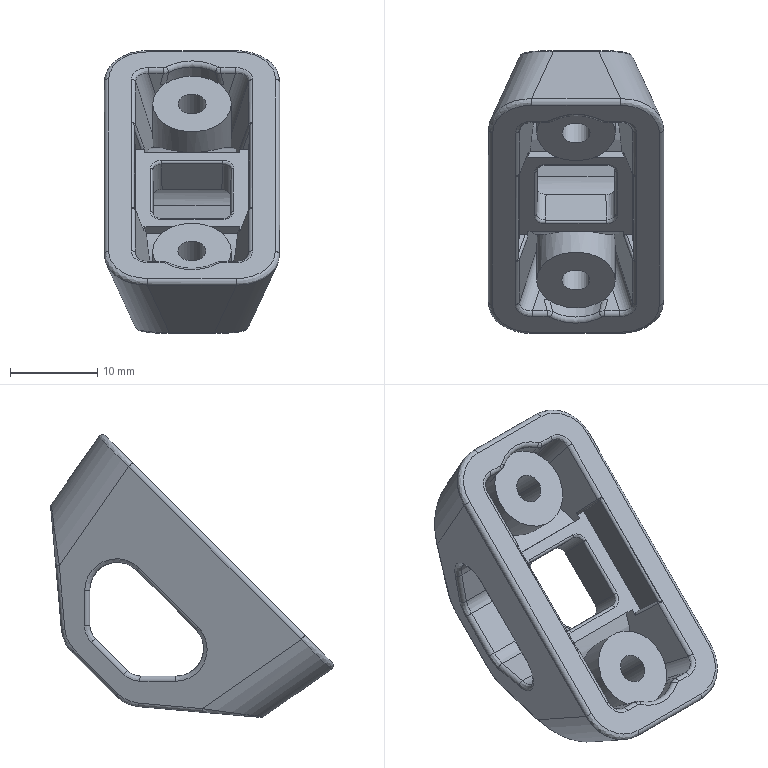Part | SolidWorks | features BaseBody 1 | 1 solid | 149 faces | box 20.093 x 32.379 x 32.401 mm | volume 5600 mm3 | cylinder 70 | spline 40 | plane 37 | torus 2 | commonest cylinder face diameters 1 x26 0.6 x12 9 x8 2 x4 3 x4 3.2 x4